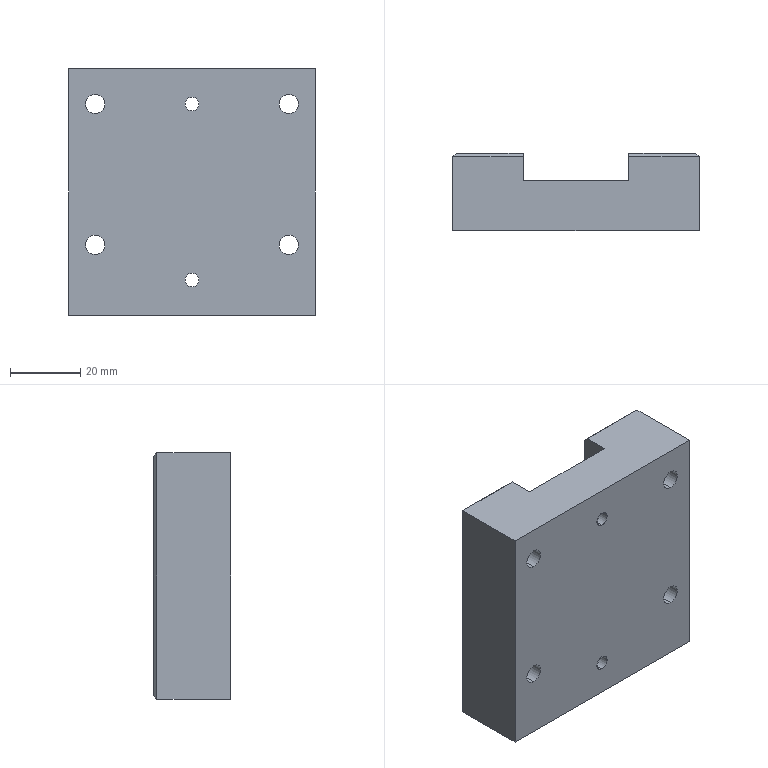Part | STEP file | PN_0020 Connecting plate | 1 solid | 44 faces | box 70 x 22 x 70 mm | volume 86429 mm3 | cylinder 20 | plane 20 | cone 4 | commonest cylinder face diameters 5.5 x8 10 x8 4.2 x4